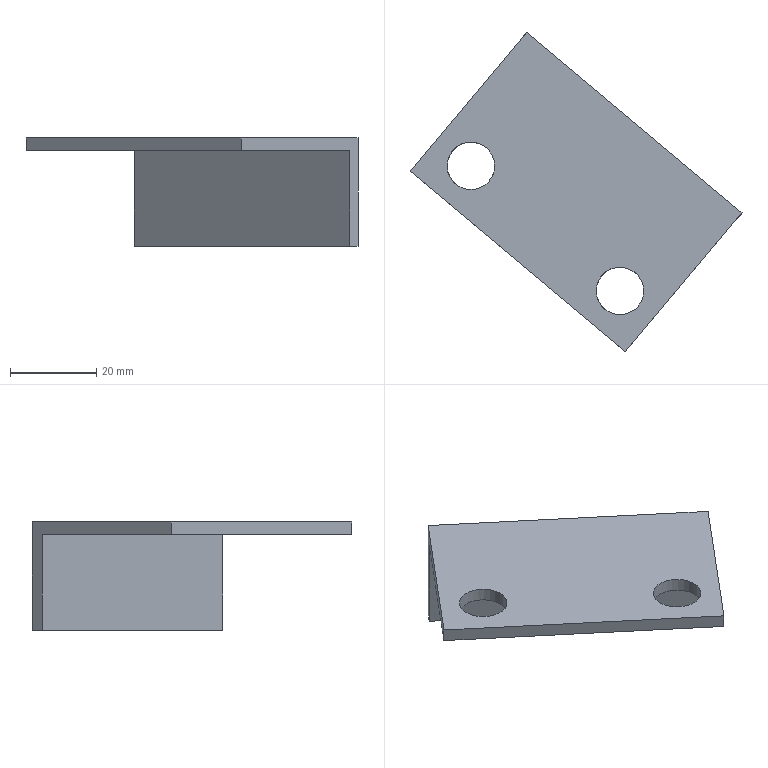Part | NX | features solid 2 | 1 solid | 10 faces | box 76.79 x 73.955 x 25 mm | volume 11910 mm3 | plane 8 | cylinder 2 | commonest cylinder face diameters 11 x2
STEP:
#1=CARTESIAN_POINT('',(692.706,739.172,127.));
#2=VERTEX_POINT('',#1);
#3=CARTESIAN_POINT('',(698.206,739.172,127.));
#4=DIRECTION('',(0.,0.,-1.));
#5=DIRECTION('',(-1.,0.,0.));
#6=AXIS2_PLACEMENT_3D('',#3,#4,#5);
#7=CIRCLE('',#6,5.5);
#8=EDGE_CURVE('',#2,#2,#7,.T.);
#9=ORIENTED_EDGE('',*,*,#8,.F.);
#10=EDGE_LOOP('',(#9));
#11=FACE_BOUND('',#10,.T.);
#12=CARTESIAN_POINT('',(727.178,710.247,127.));
#13=VERTEX_POINT('',#12);
#14=CARTESIAN_POINT('',(732.678,710.247,127.));
#15=DIRECTION('',(0.,0.,-1.));
#16=DIRECTION('',(-1.,0.,0.));
#17=AXIS2_PLACEMENT_3D('',#14,#15,#16);
#18=CIRCLE('',#17,5.5);
#19=EDGE_CURVE('',#13,#13,#18,.T.);
#20=ORIENTED_EDGE('',*,*,#19,.F.);
#21=EDGE_LOOP('',(#20));
#22=FACE_BOUND('',#21,.T.);
#23=CARTESIAN_POINT('',(709.187,767.815,127.));
#24=VERTEX_POINT('',#23);
#25=CARTESIAN_POINT('',(758.98,726.034,127.));
#26=VERTEX_POINT('',#25);
#27=CARTESIAN_POINT('',(716.273,761.87,127.));
#28=DIRECTION('',(0.766,-0.6428,0.));
#29=VECTOR('',#28,1000.);
#30=LINE('',#27,#29);
#31=EDGE_CURVE('',#24,#26,#30,.T.);
#32=ORIENTED_EDGE('',*,*,#31,.T.);
#33=CARTESIAN_POINT('',(733.911,696.158,127.));
#34=VERTEX_POINT('',#33);
#35=CARTESIAN_POINT('',(760.908,728.332,127.));
#36=DIRECTION('',(-0.6428,-0.766,0.));
#37=VECTOR('',#36,1000.);
#38=LINE('',#35,#37);
#39=EDGE_CURVE('',#26,#34,#38,.T.);
#40=ORIENTED_EDGE('',*,*,#39,.T.);
#41=CARTESIAN_POINT('',(684.118,737.94,127.));
#42=VERTEX_POINT('',#41);
#43=CARTESIAN_POINT('',(691.204,731.994,127.));
#44=DIRECTION('',(0.766,-0.6428,0.));
#45=VECTOR('',#44,1000.);
#46=LINE('',#43,#45);
#47=EDGE_CURVE('',#42,#34,#46,.T.);
#48=ORIENTED_EDGE('',*,*,#47,.F.);
#49=CARTESIAN_POINT('',(711.115,770.113,127.));
#50=DIRECTION('',(-0.6428,-0.766,0.));
#51=VECTOR('',#50,1000.);
#52=LINE('',#49,#51);
#53=EDGE_CURVE('',#24,#42,#52,.T.);
#54=ORIENTED_EDGE('',*,*,#53,.F.);
#55=EDGE_LOOP('',(#32,#40,#48,#54));
#56=FACE_BOUND('',#55,.T.);
#57=CARTESIAN_POINT('',(718.201,764.168,127.));
#58=DIRECTION('',(0.,0.,1.));
#59=DIRECTION('',(0.766,-0.6428,0.));
#60=AXIS2_PLACEMENT_3D('',#57,#58,#59);
#61=PLANE('',#60);
#62=ADVANCED_FACE('',(#11,#22,#56),#61,.F.);
#63=CARTESIAN_POINT('',(760.908,728.332,130.));
#64=VERTEX_POINT('',#63);
#65=CARTESIAN_POINT('',(760.908,728.332,105.));
#66=VERTEX_POINT('',#65);
#67=CARTESIAN_POINT('',(760.908,728.332,130.));
#68=DIRECTION('',(0.,0.,-1.));
#69=VECTOR('',#68,1000.);
#70=LINE('',#67,#69);
#71=EDGE_CURVE('',#64,#66,#70,.T.);
#72=ORIENTED_EDGE('',*,*,#71,.F.);
#73=CARTESIAN_POINT('',(733.911,696.158,130.));
#74=VERTEX_POINT('',#73);
#75=CARTESIAN_POINT('',(760.908,728.332,130.));
#76=DIRECTION('',(-0.6428,-0.766,0.));
#77=VECTOR('',#76,1000.);
#78=LINE('',#75,#77);
#79=EDGE_CURVE('',#64,#74,#78,.T.);
#80=ORIENTED_EDGE('',*,*,#79,.T.);
#81=CARTESIAN_POINT('',(733.911,696.158,130.));
#82=DIRECTION('',(0.,0.,-1.));
#83=VECTOR('',#82,1000.);
#84=LINE('',#81,#83);
#85=EDGE_CURVE('',#74,#34,#84,.T.);
#86=ORIENTED_EDGE('',*,*,#85,.T.);
#87=ORIENTED_EDGE('',*,*,#39,.F.);
#88=CARTESIAN_POINT('',(758.98,726.034,105.));
#89=VERTEX_POINT('',#88);
#90=CARTESIAN_POINT('',(758.98,726.034,94.));
#91=DIRECTION('',(0.,0.,1.));
#92=VECTOR('',#91,1000.);
#93=LINE('',#90,#92);
#94=EDGE_CURVE('',#89,#26,#93,.T.);
#95=ORIENTED_EDGE('',*,*,#94,.F.);
#96=CARTESIAN_POINT('',(760.908,728.332,105.));
#97=DIRECTION('',(-0.6428,-0.766,0.));
#98=VECTOR('',#97,1000.);
#99=LINE('',#96,#98);
#100=EDGE_CURVE('',#66,#89,#99,.T.);
#101=ORIENTED_EDGE('',*,*,#100,.F.);
#102=EDGE_LOOP('',(#72,#80,#86,#87,#95,#101));
#103=FACE_BOUND('',#102,.T.);
#104=CARTESIAN_POINT('',(760.908,728.332,130.));
#105=DIRECTION('',(0.766,-0.6428,0.));
#106=DIRECTION('',(0.6428,0.766,0.));
#107=AXIS2_PLACEMENT_3D('',#104,#105,#106);
#108=PLANE('',#107);
#109=ADVANCED_FACE('',(#103),#108,.T.);
#110=CARTESIAN_POINT('',(702.42,735.637,130.));
#111=VERTEX_POINT('',#110);
#112=CARTESIAN_POINT('',(698.206,739.172,130.));
#113=DIRECTION('',(0.,0.,-1.));
#114=DIRECTION('',(0.766,-0.6428,0.));
#115=AXIS2_PLACEMENT_3D('',#112,#113,#114);
#116=CIRCLE('',#115,5.5);
#117=EDGE_CURVE('',#111,#111,#116,.T.);
#118=ORIENTED_EDGE('',*,*,#117,.T.);
#119=EDGE_LOOP('',(#118));
#120=FACE_BOUND('',#119,.T.);
#121=CARTESIAN_POINT('',(736.892,706.711,130.));
#122=VERTEX_POINT('',#121);
#123=CARTESIAN_POINT('',(732.678,710.247,130.));
#124=DIRECTION('',(0.,0.,-1.));
#125=DIRECTION('',(0.766,-0.6428,0.));
#126=AXIS2_PLACEMENT_3D('',#123,#124,#125);
#127=CIRCLE('',#126,5.5);
#128=EDGE_CURVE('',#122,#122,#127,.T.);
#129=ORIENTED_EDGE('',*,*,#128,.T.);
#130=EDGE_LOOP('',(#129));
#131=FACE_BOUND('',#130,.T.);
#132=ORIENTED_EDGE('',*,*,#79,.F.);
#133=CARTESIAN_POINT('',(711.115,770.113,130.));
#134=VERTEX_POINT('',#133);
#135=CARTESIAN_POINT('',(718.201,764.168,130.));
#136=DIRECTION('',(0.766,-0.6428,0.));
#137=VECTOR('',#136,1000.);
#138=LINE('',#135,#137);
#139=EDGE_CURVE('',#134,#64,#138,.T.);
#140=ORIENTED_EDGE('',*,*,#139,.F.);
#141=CARTESIAN_POINT('',(684.118,737.94,130.));
#142=VERTEX_POINT('',#141);
#143=CARTESIAN_POINT('',(711.115,770.113,130.));
#144=DIRECTION('',(-0.6428,-0.766,0.));
#145=VECTOR('',#144,1000.);
#146=LINE('',#143,#145);
#147=EDGE_CURVE('',#134,#142,#146,.T.);
#148=ORIENTED_EDGE('',*,*,#147,.T.);
#149=CARTESIAN_POINT('',(691.204,731.994,130.));
#150=DIRECTION('',(0.766,-0.6428,0.));
#151=VECTOR('',#150,1000.);
#152=LINE('',#149,#151);
#153=EDGE_CURVE('',#142,#74,#152,.T.);
#154=ORIENTED_EDGE('',*,*,#153,.T.);
#155=EDGE_LOOP('',(#132,#140,#148,#154));
#156=FACE_BOUND('',#155,.T.);
#157=CARTESIAN_POINT('',(718.201,764.168,130.));
#158=DIRECTION('',(0.,0.,1.));
#159=DIRECTION('',(0.766,-0.6428,0.));
#160=AXIS2_PLACEMENT_3D('',#157,#158,#159);
#161=PLANE('',#160);
#162=ADVANCED_FACE('',(#120,#131,#156),#161,.T.);
#163=ORIENTED_EDGE('',*,*,#147,.F.);
#164=CARTESIAN_POINT('',(711.115,770.113,105.));
#165=VERTEX_POINT('',#164);
#166=CARTESIAN_POINT('',(711.115,770.113,130.));
#167=DIRECTION('',(0.,0.,-1.));
#168=VECTOR('',#167,1000.);
#169=LINE('',#166,#168);
#170=EDGE_CURVE('',#134,#165,#169,.T.);
#171=ORIENTED_EDGE('',*,*,#170,.T.);
#172=CARTESIAN_POINT('',(709.187,767.815,105.));
#173=VERTEX_POINT('',#172);
#174=CARTESIAN_POINT('',(711.115,770.113,105.));
#175=DIRECTION('',(-0.6428,-0.766,0.));
#176=VECTOR('',#175,1000.);
#177=LINE('',#174,#176);
#178=EDGE_CURVE('',#165,#173,#177,.T.);
#179=ORIENTED_EDGE('',*,*,#178,.T.);
#180=CARTESIAN_POINT('',(709.187,767.815,94.));
#181=DIRECTION('',(0.,0.,1.));
#182=VECTOR('',#181,1000.);
#183=LINE('',#180,#182);
#184=EDGE_CURVE('',#173,#24,#183,.T.);
#185=ORIENTED_EDGE('',*,*,#184,.T.);
#186=ORIENTED_EDGE('',*,*,#53,.T.);
#187=CARTESIAN_POINT('',(684.118,737.94,130.));
#188=DIRECTION('',(0.,0.,-1.));
#189=VECTOR('',#188,1000.);
#190=LINE('',#187,#189);
#191=EDGE_CURVE('',#142,#42,#190,.T.);
#192=ORIENTED_EDGE('',*,*,#191,.F.);
#193=EDGE_LOOP('',(#163,#171,#179,#185,#186,#192));
#194=FACE_BOUND('',#193,.T.);
#195=CARTESIAN_POINT('',(711.115,770.113,57.5));
#196=DIRECTION('',(0.766,-0.6428,0.));
#197=DIRECTION('',(0.,0.,-1.));
#198=AXIS2_PLACEMENT_3D('',#195,#196,#197);
#199=PLANE('',#198);
#200=ADVANCED_FACE('',(#194),#199,.F.);
#201=ORIENTED_EDGE('',*,*,#170,.F.);
#202=ORIENTED_EDGE('',*,*,#139,.T.);
#203=ORIENTED_EDGE('',*,*,#71,.T.);
#204=CARTESIAN_POINT('',(709.2,771.72,105.));
#205=DIRECTION('',(0.766,-0.6428,0.));
#206=VECTOR('',#205,1000.);
#207=LINE('',#204,#206);
#208=EDGE_CURVE('',#165,#66,#207,.T.);
#209=ORIENTED_EDGE('',*,*,#208,.F.);
#210=EDGE_LOOP('',(#201,#202,#203,#209));
#211=FACE_BOUND('',#210,.T.);
#212=CARTESIAN_POINT('',(718.201,764.168,130.));
#213=DIRECTION('',(-0.6428,-0.766,0.));
#214=DIRECTION('',(0.766,-0.6428,0.));
#215=AXIS2_PLACEMENT_3D('',#212,#213,#214);
#216=PLANE('',#215);
#217=ADVANCED_FACE('',(#211),#216,.F.);
#218=ORIENTED_EDGE('',*,*,#47,.T.);
#219=ORIENTED_EDGE('',*,*,#85,.F.);
#220=ORIENTED_EDGE('',*,*,#153,.F.);
#221=ORIENTED_EDGE('',*,*,#191,.T.);
#222=EDGE_LOOP('',(#218,#219,#220,#221));
#223=FACE_BOUND('',#222,.T.);
#224=CARTESIAN_POINT('',(691.204,731.994,130.));
#225=DIRECTION('',(-0.6428,-0.766,0.));
#226=DIRECTION('',(0.766,-0.6428,0.));
#227=AXIS2_PLACEMENT_3D('',#224,#225,#226);
#228=PLANE('',#227);
#229=ADVANCED_FACE('',(#223),#228,.T.);
#230=ORIENTED_EDGE('',*,*,#184,.F.);
#231=CARTESIAN_POINT('',(707.272,769.422,105.));
#232=DIRECTION('',(0.766,-0.6428,0.));
#233=VECTOR('',#232,1000.);
#234=LINE('',#231,#233);
#235=EDGE_CURVE('',#173,#89,#234,.T.);
#236=ORIENTED_EDGE('',*,*,#235,.T.);
#237=ORIENTED_EDGE('',*,*,#94,.T.);
#238=ORIENTED_EDGE('',*,*,#31,.F.);
#239=EDGE_LOOP('',(#230,#236,#237,#238));
#240=FACE_BOUND('',#239,.T.);
#241=CARTESIAN_POINT('',(707.272,769.422,94.));
#242=DIRECTION('',(0.6428,0.766,0.));
#243=DIRECTION('',(-0.766,0.6428,0.));
#244=AXIS2_PLACEMENT_3D('',#241,#242,#243);
#245=PLANE('',#244);
#246=ADVANCED_FACE('',(#240),#245,.F.);
#247=ORIENTED_EDGE('',*,*,#100,.T.);
#248=ORIENTED_EDGE('',*,*,#235,.F.);
#249=ORIENTED_EDGE('',*,*,#178,.F.);
#250=ORIENTED_EDGE('',*,*,#208,.T.);
#251=EDGE_LOOP('',(#247,#248,#249,#250));
#252=FACE_BOUND('',#251,.T.);
#253=CARTESIAN_POINT('',(709.2,771.72,105.));
#254=DIRECTION('',(0.,0.,-1.));
#255=DIRECTION('',(0.766,-0.6428,0.));
#256=AXIS2_PLACEMENT_3D('',#253,#254,#255);
#257=PLANE('',#256);
#258=ADVANCED_FACE('',(#252),#257,.T.);
#259=ORIENTED_EDGE('',*,*,#128,.F.);
#260=EDGE_LOOP('',(#259));
#261=FACE_BOUND('',#260,.T.);
#262=ORIENTED_EDGE('',*,*,#19,.T.);
#263=EDGE_LOOP('',(#262));
#264=FACE_BOUND('',#263,.T.);
#265=CARTESIAN_POINT('',(732.678,710.247,126.8));
#266=DIRECTION('',(0.,0.,1.));
#267=DIRECTION('',(0.766,-0.6428,0.));
#268=AXIS2_PLACEMENT_3D('',#265,#266,#267);
#269=CYLINDRICAL_SURFACE('',#268,5.5);
#270=ADVANCED_FACE('',(#261,#264),#269,.F.);
#271=ORIENTED_EDGE('',*,*,#117,.F.);
#272=EDGE_LOOP('',(#271));
#273=FACE_BOUND('',#272,.T.);
#274=ORIENTED_EDGE('',*,*,#8,.T.);
#275=EDGE_LOOP('',(#274));
#276=FACE_BOUND('',#275,.T.);
#277=CARTESIAN_POINT('',(698.206,739.172,126.8));
#278=DIRECTION('',(0.,0.,1.));
#279=DIRECTION('',(0.766,-0.6428,0.));
#280=AXIS2_PLACEMENT_3D('',#277,#278,#279);
#281=CYLINDRICAL_SURFACE('',#280,5.5);
#282=ADVANCED_FACE('',(#273,#276),#281,.F.);
#283=CLOSED_SHELL('',(#62,#109,#162,#200,#217,#229,#246,#258,#270,#282));
#284=MANIFOLD_SOLID_BREP('',#283);
#285=(LENGTH_UNIT()NAMED_UNIT(*)SI_UNIT(.MILLI.,.METRE.));
#286=UNCERTAINTY_MEASURE_WITH_UNIT(LENGTH_MEASURE(0.00001),#285,'','');
#287=(NAMED_UNIT(*)PLANE_ANGLE_UNIT()SI_UNIT($,.RADIAN.));
#288=(NAMED_UNIT(*)SI_UNIT($,.STERADIAN.)SOLID_ANGLE_UNIT());
#289=(GEOMETRIC_REPRESENTATION_CONTEXT(3)GLOBAL_UNCERTAINTY_ASSIGNED_CONTEXT((#286))GLOBAL_UNIT_ASSIGNED_CONTEXT((#285,#287,#288))REPRESENTATION_CONTEXT('',''));
#290=ADVANCED_BREP_SHAPE_REPRESENTATION('',(#284),#289);